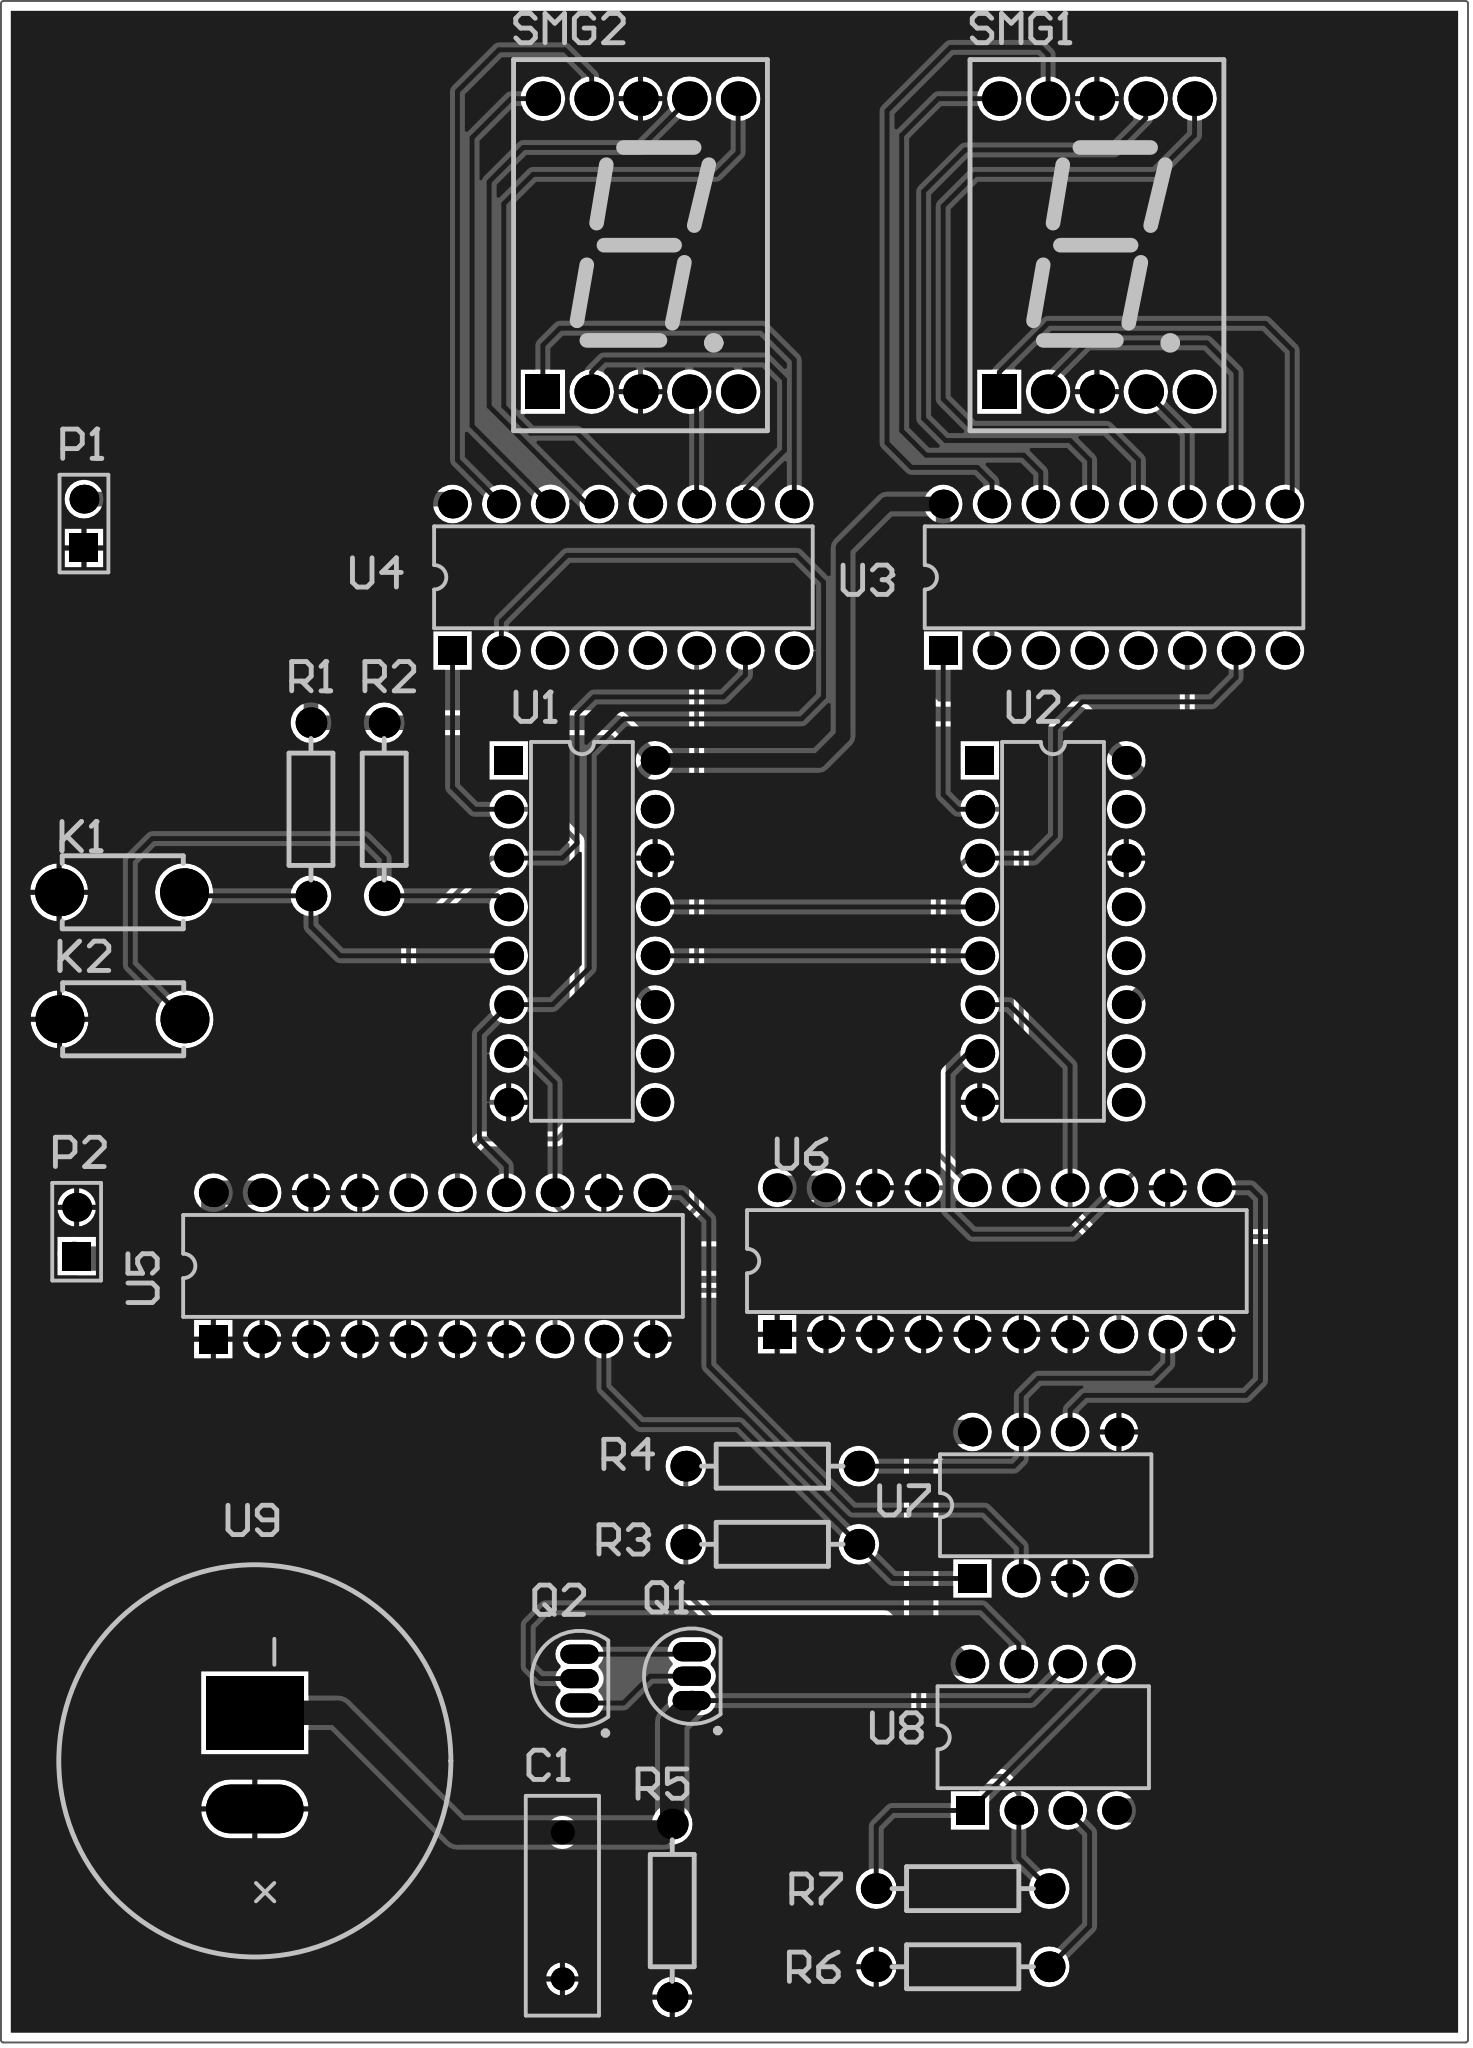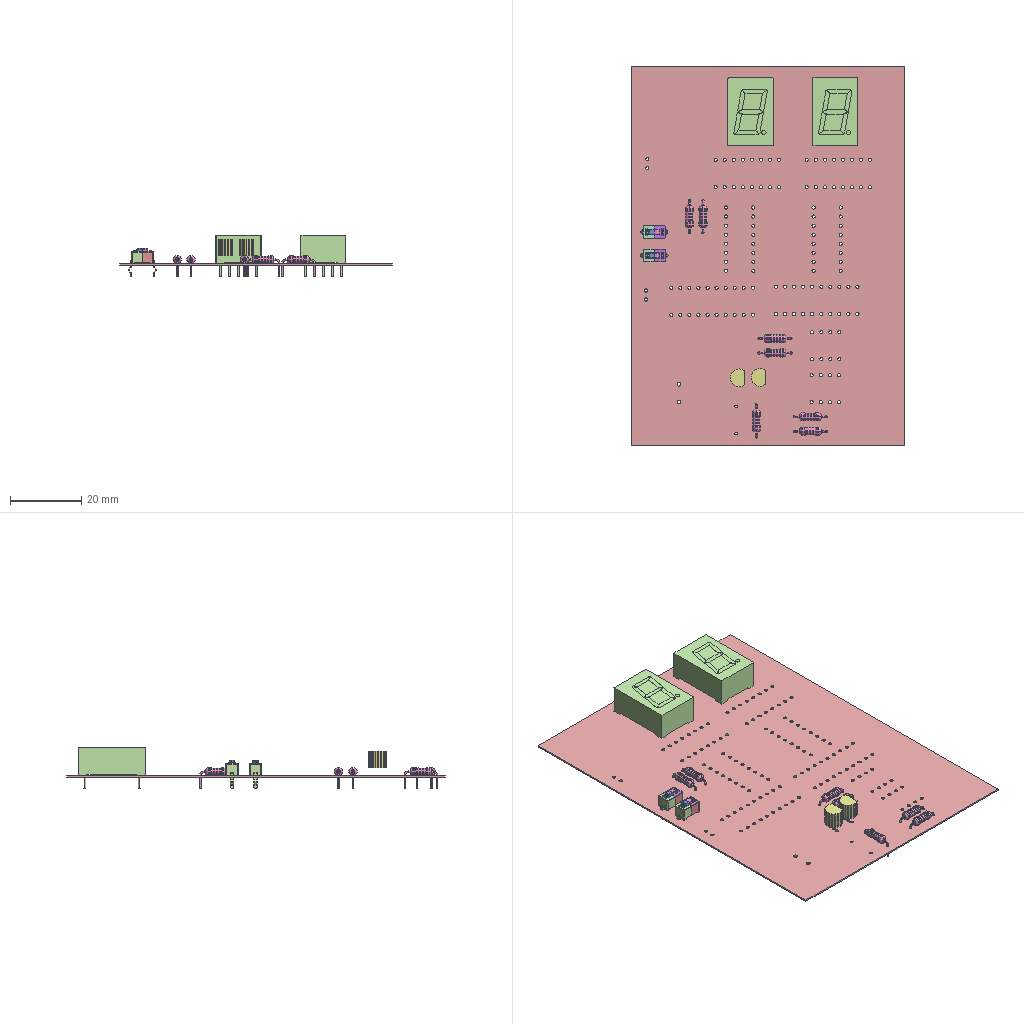Circuit board layout | Altium Designer | box 76.3 x 106.2 x 11.6 mm
Layer stack:
# Altium Designer layer stack of  (unit mm; dielectric type: 0 none, 1 core, 2 prepreg, 3 surface material)
index,name,kind,layer,copper_thickness_mm,dielectric_type,dielectric_thickness_mm,dielectric_material,dielectric_constant
0,Top Paste,other,,,,,,
1,Top Overlay,other,,,,,,
2,Top Solder,dielectric,,,3,0.0102,Solder Resist,3.5
3,Top Layer,copper,Top Layer,0.0356,,,,
4,Dielectric 1,dielectric,,,0,0.32,FR-4,4.8
5,Bottom Layer,copper,Bottom Layer,0.0356,,,,
6,Bottom Solder,dielectric,,,3,0.0102,Solder Resist,3.5
7,Bottom Overlay,other,,,,,,
8,Bottom Paste,other,,,,,,
# drill layer pairs: low layer,high layer
drill_pair,Top Layer,Bottom Layer
Part placement:
Designator,Comment,Layer,Footprint,Center-X(mm),Center-Y(mm),Rotation
U9,Volts,TopLayer,CAPACITANCE_1_FARAD_5,5_VOLT,99.568,39.41,90
U8,NE5532,TopLayer,P008,140.589,40.64,0
U7,NE5532,TopLayer,P008,140.716,52.705,0
U6,DAC0832,TopLayer,J20A,138.176,65.405,360
U5,DAC0832,TopLayer,J20A,108.839,65.151,360
U4,SN74LS48N,TopLayer,N016D,118.745,100.965,360
U3,SN74LS48N,TopLayer,N016D,144.272,100.965,360
U2,SN74LS192N,TopLayer,648-08,141.097,82.55,270
U1,SN74LS192N,TopLayer,648-08,116.586,82.55,270
SMG2,5011A,TopLayer,SMG_0.5-1P,119.634,118.237,0
SMG1,5011A,TopLayer,SMG_0.5-1P,143.383,118.237,0
R7,10K,TopLayer,RS_1/4W,136.398,32.766,180
R6,10K,TopLayer,RS_1/4W,136.398,28.702,360
R5,10K,TopLayer,RS_1/4W,121.285,31.623,270
R4,10K,TopLayer,RS_1/4W,126.492,54.737,360
R3,100K,TopLayer,RS_1/4W,126.492,50.673,360
R2,10K,TopLayer,RS_1/4W,106.299,88.9,90
R1,10K,TopLayer,RS_1/4W,102.489,88.9,90
Q2,2N3904,TopLayer,TO-92A,116.459,43.688,0
Q1,2N3055,TopLayer,TO-92A,122.301,43.815,0
P2,Header 2,TopLayer,HDR1X2,90.297,66.929,90
P1,Header 2,TopLayer,HDR1X2,90.678,103.759,90
K2,KEY,TopLayer,DIP-3X6X4.3,92.658,77.978,360
K1,KEY,TopLayer,DIP-3X6X4.3,92.635,84.582,360
C1,100UF,TopLayer,RAD-0.3,115.57,31.877,90
Pad and via stacks:
# Altium Designer via and pad stacks of  (unit mm). Each distinct definition once, with the count of objects using it.
# via: kind,start_layer,end_layer,hole_mm,diameter_mm,mode(0 simple;1 top-mid-bottom;2 full stack),diameter_per_layer,count,example_net
# pad: kind,layer,hole_mm,hole_type(0 round;1 square;2 slot),plating,top_size,top_shape(1 round;2 rect;3 octagon;9 rounded rect),mid_size,bottom_size,mode,footprint,size_per_layer,count,example
pad,Multi-Layer,0.9,0,plated,1.5x1.5,1,1.5x1.5,1.5x1.5,0,648-08,,30,U1.9
pad,Multi-Layer,0.9,0,plated,1.5x1.5,2,1.5x1.5,1.5x1.5,0,648-08,,2,U1.1
pad,Multi-Layer,0.6,0,plated,1.6x1.6,1,1.6x1.6,1.6x1.6,0,RS 1/4W,,14,R2.2
pad,Multi-Layer,0.9,0,plated,1.5x1.5,1,1.5x1.5,1.5x1.5,0,N016D,,30,U4.9
pad,Multi-Layer,0.9,0,plated,1.5x1.5,2,1.5x1.5,1.5x1.5,0,N016D,,2,U4.1
pad,Multi-Layer,1.2,0,plated,2.5x2.5,1,2.5x2.5,2.5x2.5,0,DIP-3X6X4.3,,4,K1.1
pad,Multi-Layer,0.9,0,plated,1.8x1.8,2,1.8x1.8,1.8x1.8,0,SMG 0.5-1P,,2,SMG2.1
pad,Multi-Layer,0.9,0,plated,1.8x1.8,1,1.8x1.8,1.8x1.8,0,SMG 0.5-1P,,18,SMG2.2
pad,Multi-Layer,0.9,0,plated,1.5x1.5,1,1.5x1.5,1.5x1.5,0,J20A,,38,U6.11
pad,Multi-Layer,0.9,0,plated,1.5x1.5,2,1.5x1.5,1.5x1.5,0,J20A,,2,U6.1
pad,Multi-Layer,0.9,0,plated,1.5x1.5,2,1.5x1.5,1.5x1.5,0,HDR1X2,,2,P2.1
pad,Multi-Layer,0.9,0,plated,1.5x1.5,1,1.5x1.5,1.5x1.5,0,HDR1X2,,2,P2.2
pad,Multi-Layer,0.9,0,plated,1.5x1.5,2,1.5x1.5,1.5x1.5,0,P008,,2,U7.1
pad,Multi-Layer,0.9,0,plated,1.5x1.5,1,1.5x1.5,1.5x1.5,0,P008,,14,U7.2
pad,Multi-Layer,0.9,0,plated,2x1,1,2x1,2x1,0,TO-92A,,6,Q1.3
pad,Multi-Layer,1.1,0,plated,3.81x5.08,2,3.81x5.08,3.81x5.08,0,CAPACITANCE 1 FARAD 5,5 VOLT,,1,U9.1
pad,Multi-Layer,1.1,0,plated,2.54x5.08,1,2.54x5.08,2.54x5.08,0,CAPACITANCE 1 FARAD 5,5 VOLT,,1,U9.2
pad,Multi-Layer,0.7,0,plated,1.2x1.2,1,1.2x1.2,1.2x1.2,0,RAD-0.3,,2,C1.2
Copper pours:
name,layer,net,type(0 solid;1 hatched;2 none)
D,Bottom Layer,GND,0
D,Top Layer,GND,0
Design rules, without the lines most boards share:
# Altium Designer design rules of  (exported by Altium Designer, unit mm)
# columns: name | kind | enabled | priority | scope1 | scope2 | descriptor | typed fields (field=value)
SilkToSilkClearance | 55 | enabled | 1 | All | All | Silk to Silk (Clearance=0mil) (All),(All) |
SilkToSolderMaskClearance | 54 | enabled | 1 | IsPad | All | Silk To Solder Mask (Clearance=0mil) (IsPad),(All) |
MinimumSolderMaskSliver | 53 | enabled | 1 | All | All | Minimum Solder Mask Sliver (Gap=0mil) (All),(All) |
HoleToHoleClearance | 52 | enabled | 1 | All | All | Hole To Hole Clearance (Gap=10mil) (All),(All) | gap=0.254
DiffPairsRouting | 51 | enabled | 1 | All | All | Differential Pairs Uncoupled Length using the Gap Constraints (Min=10mil) (Max=10mil) (Prefered=10mil)  and Width Constraints (Min=15mil) (Max=15mil) (Prefered=15mil) (All) |
HoleSize | 42 | enabled | 1 | All | All | Hole Size Constraint (Min=1mil) (Max=99999mil) (All) |
SolderMaskExpansion | 13 | enabled | 1 | All | All | Solder Mask Expansion (Expansion =4mil) (All) | expansion=0.1016
PasteMaskExpansion | 14 | enabled | 1 | All | All | Paste Mask Expansion (Expansion =0mil) (All) | expansion=0
RoutingVias | 11 | enabled | 1 | All | All | Routing Via (MinHoleWidth=28mil) (MaxHoleWidth=28mil) (PreferredHoleWidth=28mil) (MinWidth=50mil) (MaxWidth=50mil) (PreferedWidth=50mil) (All) | via_min_hole=0.7112 via_max_hole=0.7112 via_preferred_diameter=1.27 via_preferred_hole=0.7112
Width | 2 | enabled | 1 | All | All | Width Constraint (Min=10mil) (Max=50mil) (Preferred=10mil) (All) |
PolygonConnect | 20 | enabled | 1 | All | All | Polygon Connect Rule(Relief Connect )(Conductor Width=10mil) (Relief Angle=90 Angle) (Entries=4) (Air Gap Width=10mil) (All),(All) | connect_style(0=relief,1=direct,2=none)=0 relief_conductor_width=0.254 relief_entries=4
PlaneConnect | 6 | enabled | 1 | All | All | Power Plane Connect Rule(Relief Connect )(Expansion=20mil) (Conductor Width=10mil) (Air Gap=10mil) (Entries=4) (All) | relief_conductor_width=0.254 relief_entries=4 relief_expansion=0.508
Clearance | 0 | enabled | 1 | All | All | Clearance Constraint (Gap=10mil) (All),(All) | gap=0.254
Classes set for this board:
# Altium Designer classes of  (member kind: 0 net, 1 component, 2 from-to, 3 pad, 4 layer, 5 differential pair, 6 design channel, 7 polygon, 8 structure, 9 xSignal)
# columns: class name | member kind | superclass | members
Sheet1 | 1 | no | C1; K1; K2; P1; P2; Q1; Q2; R1; R2; R3; R4; R5; R6; R7; SMG1; SMG2; U1; U2; U3; U4; U5; U6; U7; U8; U9;